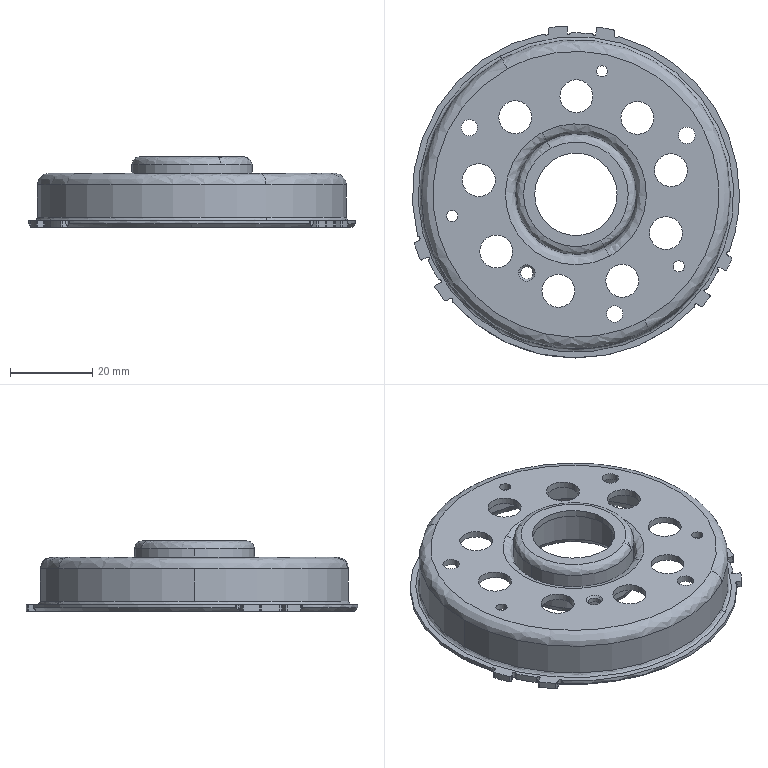Part | STEP file | TQ-DD-1105-THBrg.Holder(A140059500A)1010_デフォルト | 1 solid | 144 faces | box 79.4 x 80.57 x 17.1 mm | volume 12458 mm3 | cylinder 101 | spline 18 | plane 18 | cone 7 | commonest cylinder face diameters 8 x18 0.6 x14 0.8 x14 0.738 x8 1.01 x6 2.7 x6